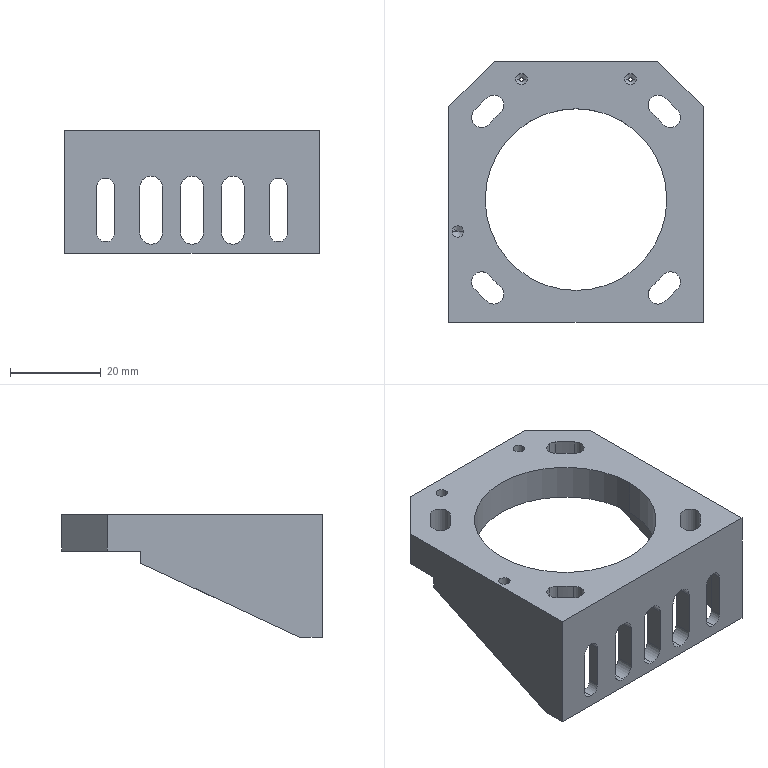NC program | NX | posted with a generic post | part box 56 x 57.4 x 27 mm
Lines 13891 to 14809 of 23725:
(ZLEVEL_PROFILE_COPY_2 , TOOL : D6JING)
N27762 T06 M6
N27764 G54
N27766 G17 G0 G90 X-22. Y20.857 B0. C0. S5000 M3
N27768 G43 Z30. H6
N27770 Z-0.1
N27772 G94 G1 X-22.627 Y21.749 F1000.
N27774 G3 X-23.171 Y22.001 R0.6
N27776 G1 X-23.2 Y21.999 F1500.
N27778 Y20.313
N27780 G3 X-22.9 Y19.793 R0.6
N27782 G1 X-22. Y19.274
N27784 G0 Y20.767 Z-0.2
N27786 G1 X-22.639 Y21.732 F1000.
N27788 G3 X-23.176 Y22. R0.6
N27790 G1 X-23.2 Y21.999 F1500.
N27792 Y20.227
N27794 G3 X-22.9 Y19.707 R0.6
N27796 G1 X-22. Y19.188
N27798 G0 Y20.77 Z-0.3
N27800 G1 X-22.537 Y21.7 F1000.
N27802 G3 X-23.057 Y22. R0.6
N27804 G1 X-23.176 F1500.
N27806 X-23.2 Y21.999
N27808 Y20.14
N27810 G3 X-22.9 Y19.621 R0.6
N27812 G1 X-22. Y19.101
N27814 G0 X-21.87 Y20.917 Z-0.4
N27816 G1 X-22.323 Y21.7 F1000.
N27818 G3 X-22.842 Y22. R0.6
N27820 G1 X-23.176 F1500.
N27822 X-23.2 Y21.999
N27824 Y20.061
N27826 G3 X-22.9 Y19.541 R0.6
N27828 G1 X-22. Y19.021
N27830 G0 X-21.654 Y20.914 Z-0.5
N27832 G1 X-22.108 Y21.7 F1000.
N27834 G3 X-22.628 Y22. R0.6
N27836 G1 X-23.176 F1500.
N27838 X-23.2 Y21.999
N27840 Y19.993
N27842 G3 X-22.9 Y19.474 R0.6
N27844 G1 X-22. Y18.954
N27846 G0 X-21.44 Y20.914 Z-0.6
N27848 G1 X-21.894 Y21.7 F1000.
N27850 G3 X-22.413 Y22. R0.6
N27852 G1 X-23.176 F1500.
N27854 X-23.2 Y21.999
N27856 Y19.933
N27858 G3 X-22.9 Y19.414 R0.6
N27860 G1 X-22. Y18.894
N27862 G0 X-21.226 Y20.914 Z-0.7
N27864 G1 X-21.679 Y21.7 F1000.
N27866 G3 X-22.199 Y22. R0.6
N27868 G1 X-23.176 F1500.
N27870 X-23.2 Y21.999
N27872 Y19.885
N27874 G3 X-22.9 Y19.365 R0.6
N27876 G1 X-22. Y18.846
N27878 G0 X-21.011 Y20.914 Z-0.8
N27880 G1 X-21.465 Y21.7 F1000.
N27882 G3 X-21.984 Y22. R0.6
N27884 G1 X-23.176 F1500.
N27886 X-23.2 Y21.999
N27888 Y19.845
N27890 G3 X-22.9 Y19.326 R0.6
N27892 G1 X-22. Y18.806
N27894 G0 X-20.797 Y20.914 Z-0.9
N27896 G1 X-21.25 Y21.7 F1000.
N27898 G3 X-21.77 Y22. R0.6
N27900 G1 X-23.176 F1500.
N27902 X-23.2 Y21.998
N27904 Y19.817
N27906 G3 X-22.9 Y19.297 R0.6
N27908 G1 X-22. Y18.778
N27910 G0 X-20.582 Y20.914 Z-1.
N27912 G1 X-21.036 Y21.7 F1000.
N27914 G3 X-21.555 Y22. R0.6
N27916 G1 X-23.176 F1500.
N27918 X-23.2 Y21.998
N27920 Y19.796
N27922 G3 X-22.9 Y19.277 R0.6
N27924 G1 X-22. Y18.757
N27926 G0 X-20.368 Y20.914 Z-1.1
N27928 G1 X-20.821 Y21.7 F1000.
N27930 G3 X-21.341 Y22. R0.6
N27932 G1 X-23.176 F1500.
N27934 X-23.2 Y21.998
N27936 Y19.786
N27938 G3 X-22.9 Y19.267 R0.6
N27940 G1 X-22. Y18.747
N27942 G0 X-20.153 Y20.914 Z-1.2
N27944 G1 X-20.607 Y21.7 F1000.
N27946 G3 X-21.127 Y22. R0.6
N27948 G1 X-23.176 F1500.
N27950 X-23.2 Y21.998
N27952 Y19.784
N27954 G3 X-22.9 Y19.264 R0.6
N27956 G1 X-22. Y18.744
N27958 G0 X-20.002 Y20.9 Z-1.3
N27960 G1 X-20.464 Y21.7 F1000.
N27962 G3 X-20.984 Y22. R0.6
N27964 G1 X-23.176 F1500.
N27966 X-23.2 Y21.998
N27968 Y19.784
N27970 G3 X-22.9 Y19.264 R0.6
N27972 G1 X-22. Y18.744
N27974 G0 X-19.98 Y20.863 Z-1.4
N27976 G1 X-20.464 Y21.7 F1000.
N27978 G3 X-20.984 Y22. R0.6
N27980 G1 X-23.176 F1500.
N27982 X-23.2 Y21.998
N27984 Y19.784
N27986 G3 X-22.9 Y19.264 R0.6
N27988 G1 X-22. Y18.744
N27990 G0 X-19.963 Y20.832 Z-1.5
N27992 G1 X-20.464 Y21.7 F1000.
N27994 G3 X-20.984 Y22. R0.6
N27996 G1 X-23.176 F1500.
N27998 X-23.2 Y21.998
N28000 Y19.784
N28002 G3 X-22.9 Y19.264 R0.6
N28004 G1 X-22. Y18.744
N28006 G0 X-19.952 Y20.813 Z-1.6
N28008 G1 X-20.464 Y21.7 F1000.
N28010 G3 X-20.984 Y22. R0.6
N28012 G1 X-23.176 F1500.
N28014 X-23.2 Y21.998
N28016 Y19.784
N28018 G3 X-22.9 Y19.264 R0.6
N28020 G1 X-22. Y18.744
N28022 G0 X-19.945 Y20.802 Z-1.7
N28024 G1 X-20.464 Y21.7 F1000.
N28026 G3 X-20.984 Y22. R0.6
N28028 G1 X-23.176 F1500.
N28030 X-23.2 Y21.998
N28032 Y19.784
N28034 G3 X-22.9 Y19.264 R0.6
N28036 G1 X-22. Y18.744
N28038 G0 X-19.944 Y20.8 Z-1.8
N28040 G1 X-20.464 Y21.7 F1000.
N28042 G3 X-20.984 Y22. R0.6
N28044 G1 X-23.176 F1500.
N28046 X-23.2 Y21.998
N28048 Y19.784
N28050 G3 X-22.9 Y19.264 R0.6
N28052 G1 X-22. Y18.744
N28054 G0 X-19.944 Y20.8 Z-1.9
N28056 G1 X-20.464 Y21.7 F1000.
N28058 G3 X-20.984 Y22. R0.6
N28060 G1 X-23.176 F1500.
N28062 X-23.2 Y21.998
N28064 Y19.784
N28066 G3 X-22.9 Y19.264 R0.6
N28068 G1 X-22. Y18.744
N28070 G0 X-19.944 Y20.8 Z-2.
N28072 G1 X-20.464 Y21.7 F1000.
N28074 G3 X-20.984 Y22. R0.6
N28076 G1 X-23.176 F1500.
N28078 X-23.2 Y21.998
N28080 Y19.784
N28082 G3 X-22.9 Y19.264 R0.6
N28084 G1 X-22. Y18.744
N28086 G0 X-19.944 Y20.8 Z-2.1
N28088 G1 X-20.464 Y21.7 F1000.
N28090 G3 X-20.984 Y22. R0.6
N28092 G1 X-23.176 F1500.
N28094 X-23.2 Y21.998
N28096 Y19.784
N28098 G3 X-22.9 Y19.264 R0.6
N28100 G1 X-22. Y18.744
N28102 G0 X-19.944 Y20.8 Z-2.2
N28104 G1 X-20.464 Y21.7 F1000.
N28106 G3 X-20.984 Y22. R0.6
N28108 G1 X-23.176 F1500.
N28110 X-23.2 Y21.998
N28112 Y19.784
N28114 G3 X-22.9 Y19.264 R0.6
N28116 G1 X-22. Y18.744
N28118 G0 X-19.944 Y20.8 Z-2.3
N28120 G1 X-20.464 Y21.7 F1000.
N28122 G3 X-20.984 Y22. R0.6
N28124 G1 X-23.176 F1500.
N28126 X-23.2 Y21.998
N28128 Y19.784
N28130 G3 X-22.9 Y19.264 R0.6
N28132 G1 X-22. Y18.744
N28134 G0 X-19.944 Y20.8 Z-2.4
N28136 G1 X-20.464 Y21.7 F1000.
N28138 G3 X-20.984 Y22. R0.6
N28140 G1 X-23.176 F1500.
N28142 X-23.2 Y21.998
N28144 Y19.784
N28146 G3 X-22.9 Y19.264 R0.6
N28148 G1 X-22. Y18.744
N28150 G0 X-19.944 Y20.8 Z-2.5
N28152 G1 X-20.464 Y21.7 F1000.
N28154 G3 X-20.984 Y22. R0.6
N28156 G1 X-23.176 F1500.
N28158 X-23.2 Y21.998
N28160 Y19.784
N28162 G3 X-22.9 Y19.264 R0.6
N28164 G1 X-22. Y18.744
N28166 G0 X-19.944 Y20.8 Z-2.6
N28168 G1 X-20.464 Y21.7 F1000.
N28170 G3 X-20.984 Y22. R0.6
N28172 G1 X-23.176 F1500.
N28174 X-23.2 Y21.998
N28176 Y19.784
N28178 G3 X-22.9 Y19.264 R0.6
N28180 G1 X-22. Y18.744
N28182 G0 X-19.944 Y20.8 Z-2.7
N28184 G1 X-20.464 Y21.7 F1000.
N28186 G3 X-20.984 Y22. R0.6
N28188 G1 X-23.176 F1500.
N28190 X-23.2 Y21.998
N28192 Y19.784
N28194 G3 X-22.9 Y19.264 R0.6
N28196 G1 X-22. Y18.744
N28198 G0 X-19.944 Y20.8 Z-2.8
N28200 G1 X-20.464 Y21.7 F1000.
N28202 G3 X-20.984 Y22. R0.6
N28204 G1 X-23.176 F1500.
N28206 X-23.2 Y21.998
N28208 Y19.784
N28210 G3 X-22.9 Y19.264 R0.6
N28212 G1 X-22. Y18.744
N28214 G0 X-19.944 Y20.8 Z-2.9
N28216 G1 X-20.464 Y21.7 F1000.
N28218 G3 X-20.984 Y22. R0.6
N28220 G1 X-23.176 F1500.
N28222 X-23.2 Y21.998
N28224 Y19.784
N28226 G3 X-22.9 Y19.264 R0.6
N28228 G1 X-22. Y18.744
N28230 G0 X-19.944 Y20.8 Z-3.
N28232 G1 X-20.464 Y21.7 F1000.
N28234 G3 X-20.984 Y22. R0.6
N28236 G1 X-23.176 F1500.
N28238 X-23.2 Y21.998
N28240 Y19.784
N28242 G3 X-22.9 Y19.264 R0.6
N28244 G1 X-22. Y18.744
N28246 G0 X-19.944 Y20.8 Z-3.1
N28248 G1 X-20.464 Y21.7 F1000.
N28250 G3 X-20.984 Y22. R0.6
N28252 G1 X-23.176 F1500.
N28254 X-23.2 Y21.998
N28256 Y19.784
N28258 G3 X-22.9 Y19.264 R0.6
N28260 G1 X-22. Y18.744
N28262 G0 X-19.944 Y20.8 Z-3.2
N28264 G1 X-20.464 Y21.7 F1000.
N28266 G3 X-20.984 Y22. R0.6
N28268 G1 X-23.176 F1500.
N28270 X-23.2 Y21.998
N28272 Y19.784
N28274 G3 X-22.9 Y19.264 R0.6
N28276 G1 X-22. Y18.744
N28278 G0 X-19.944 Y20.8 Z-3.3
N28280 G1 X-20.464 Y21.7 F1000.
N28282 G3 X-20.984 Y22. R0.6
N28284 G1 X-23.176 F1500.
N28286 X-23.2 Y21.998
N28288 Y19.784
N28290 G3 X-22.9 Y19.264 R0.6
N28292 G1 X-22. Y18.744
N28294 G0 X-19.944 Y20.8 Z-3.4
N28296 G1 X-20.464 Y21.7 F1000.
N28298 G3 X-20.984 Y22. R0.6
N28300 G1 X-23.176 F1500.
N28302 X-23.2 Y21.998
N28304 Y19.784
N28306 G3 X-22.9 Y19.264 R0.6
N28308 G1 X-22. Y18.744
N28310 G0 X-19.944 Y20.8 Z-3.5
N28312 G1 X-20.464 Y21.7 F1000.
N28314 G3 X-20.984 Y22. R0.6
N28316 G1 X-23.176 F1500.
N28318 X-23.2 Y21.998
N28320 Y19.784
N28322 G3 X-22.9 Y19.264 R0.6
N28324 G1 X-22. Y18.744
N28326 G0 X-19.944 Y20.8 Z-3.6
N28328 G1 X-20.464 Y21.7 F1000.
N28330 G3 X-20.984 Y22. R0.6
N28332 G1 X-23.176 F1500.
N28334 X-23.2 Y21.998
N28336 Y19.784
N28338 G3 X-22.9 Y19.264 R0.6
N28340 G1 X-22. Y18.744
N28342 G0 X-19.944 Y20.8 Z-3.7
N28344 G1 X-20.464 Y21.7 F1000.
N28346 G3 X-20.984 Y22. R0.6
N28348 G1 X-23.176 F1500.
N28350 X-23.2 Y21.998
N28352 Y19.784
N28354 G3 X-22.9 Y19.264 R0.6
N28356 G1 X-22. Y18.744
N28358 G0 X-19.944 Y20.8 Z-3.8
N28360 G1 X-20.464 Y21.7 F1000.
N28362 G3 X-20.984 Y22. R0.6
N28364 G1 X-23.176 F1500.
N28366 X-23.2 Y21.998
N28368 Y19.784
N28370 G3 X-22.9 Y19.264 R0.6
N28372 G1 X-22. Y18.744
N28374 G0 X-19.944 Y20.8 Z-3.9
N28376 G1 X-20.464 Y21.7 F1000.
N28378 G3 X-20.984 Y22. R0.6
N28380 G1 X-23.176 F1500.
N28382 X-23.2 Y21.998
N28384 Y19.784
N28386 G3 X-22.9 Y19.264 R0.6
N28388 G1 X-22. Y18.744
N28390 G0 X-19.944 Y20.8 Z-4.
N28392 G1 X-20.464 Y21.7 F1000.
N28394 G3 X-20.984 Y22. R0.6
N28396 G1 X-23.176 F1500.
N28398 X-23.2 Y21.998
N28400 Y19.784
N28402 G3 X-22.9 Y19.264 R0.6
N28404 G1 X-22. Y18.744
N28406 G0 X-19.944 Y20.8 Z-4.1
N28408 G1 X-20.464 Y21.7 F1000.
N28410 G3 X-20.984 Y22. R0.6
N28412 G1 X-23.176 F1500.
N28414 X-23.2 Y21.998
N28416 Y19.784
N28418 G3 X-22.9 Y19.264 R0.6
N28420 G1 X-22. Y18.744
N28422 G0 X-19.944 Y20.8 Z-4.2
N28424 G1 X-20.464 Y21.7 F1000.
N28426 G3 X-20.984 Y22. R0.6
N28428 G1 X-23.176 F1500.
N28430 X-23.2 Y21.998
N28432 Y19.784
N28434 G3 X-22.9 Y19.264 R0.6
N28436 G1 X-22. Y18.744
N28438 G0 X-19.944 Y20.8 Z-4.3
N28440 G1 X-20.464 Y21.7 F1000.
N28442 G3 X-20.984 Y22. R0.6
N28444 G1 X-23.176 F1500.
N28446 X-23.2 Y21.998
N28448 Y19.784
N28450 G3 X-22.9 Y19.264 R0.6
N28452 G1 X-22. Y18.744
N28454 G0 X-19.944 Y20.8 Z-4.4
N28456 G1 X-20.464 Y21.7 F1000.
N28458 G3 X-20.984 Y22. R0.6
N28460 G1 X-23.176 F1500.
N28462 X-23.2 Y21.998
N28464 Y19.784
N28466 G3 X-22.9 Y19.264 R0.6
N28468 G1 X-22. Y18.744
N28470 G0 X-19.944 Y20.8 Z-4.5
N28472 G1 X-20.464 Y21.7 F1000.
N28474 G3 X-20.984 Y22. R0.6
N28476 G1 X-23.176 F1500.
N28478 X-23.2 Y21.998
N28480 Y19.784
N28482 G3 X-22.9 Y19.264 R0.6
N28484 G1 X-22. Y18.744
N28486 G0 X-19.944 Y20.8 Z-4.6
N28488 G1 X-20.464 Y21.7 F1000.
N28490 G3 X-20.984 Y22. R0.6
N28492 G1 X-23.176 F1500.
N28494 X-23.2 Y21.998
N28496 Y19.784
N28498 G3 X-22.9 Y19.264 R0.6
N28500 G1 X-22. Y18.744
N28502 G0 X-19.944 Y20.8 Z-4.7
N28504 G1 X-20.464 Y21.7 F1000.
N28506 G3 X-20.984 Y22. R0.6
N28508 G1 X-23.176 F1500.
N28510 X-23.2 Y21.998
N28512 Y19.784
N28514 G3 X-22.9 Y19.264 R0.6
N28516 G1 X-22. Y18.744
N28518 G0 X-19.944 Y20.8 Z-4.8
N28520 G1 X-20.464 Y21.7 F1000.
N28522 G3 X-20.984 Y22. R0.6
N28524 G1 X-23.176 F1500.
N28526 X-23.2 Y21.998
N28528 Y19.784
N28530 G3 X-22.9 Y19.264 R0.6
N28532 G1 X-22. Y18.744
N28534 G0 X-19.944 Y20.8 Z-4.9
N28536 G1 X-20.464 Y21.7 F1000.
N28538 G3 X-20.984 Y22. R0.6
N28540 G1 X-23.176 F1500.
N28542 X-23.2 Y21.998
N28544 Y19.784
N28546 G3 X-22.9 Y19.264 R0.6
N28548 G1 X-22. Y18.744
N28550 G0 X-19.944 Y20.8 Z-5.
N28552 G1 X-20.464 Y21.7 F1000.
N28554 G3 X-20.984 Y22. R0.6
N28556 G1 X-23.176 F1500.
N28558 X-23.2 Y21.998
N28560 Y19.784
N28562 G3 X-22.9 Y19.264 R0.6
N28564 G1 X-22. Y18.744
N28566 G0 X-19.944 Y20.8 Z-5.1
N28568 G1 X-20.464 Y21.7 F1000.
N28570 G3 X-20.984 Y22. R0.6
N28572 G1 X-23.176 F1500.
N28574 X-23.2 Y21.998
N28576 Y19.784
N28578 G3 X-22.9 Y19.264 R0.6
N28580 G1 X-22. Y18.744
N28582 G0 X-19.944 Y20.8 Z-5.2
N28584 G1 X-20.464 Y21.7 F1000.
N28586 G3 X-20.984 Y22. R0.6
N28588 G1 X-23.176 F1500.
N28590 X-23.2 Y21.998
N28592 Y19.784
N28594 G3 X-22.9 Y19.264 R0.6
N28596 G1 X-22. Y18.744
N28598 G0 X-19.944 Y20.8 Z-5.3
N28600 G1 X-20.464 Y21.7 F1000.
N28602 G3 X-20.984 Y22. R0.6
N28604 G1 X-23.176 F1500.
N28606 X-23.2 Y21.998
N28608 Y19.784
N28610 G3 X-22.9 Y19.264 R0.6
N28612 G1 X-22. Y18.744
N28614 G0 X-19.944 Y20.8 Z-5.4
N28616 G1 X-20.464 Y21.7 F1000.
N28618 G3 X-20.984 Y22. R0.6
N28620 G1 X-23.176 F1500.
N28622 X-23.2 Y21.998
N28624 Y19.784
N28626 G3 X-22.9 Y19.264 R0.6
N28628 G1 X-22. Y18.744
N28630 G0 X-19.944 Y20.8 Z-5.5
N28632 G1 X-20.464 Y21.7 F1000.
N28634 G3 X-20.984 Y22. R0.6
N28636 G1 X-23.176 F1500.
N28638 X-23.2 Y21.998
N28640 Y19.784
N28642 G3 X-22.9 Y19.264 R0.6
N28644 G1 X-22. Y18.744
N28646 G0 X-19.944 Y20.8 Z-5.6
N28648 G1 X-20.464 Y21.7 F1000.
N28650 G3 X-20.984 Y22. R0.6
N28652 G1 X-23.176 F1500.
N28654 X-23.2 Y21.998
N28656 Y19.784
N28658 G3 X-22.9 Y19.264 R0.6
N28660 G1 X-22. Y18.744
N28662 G0 X-19.944 Y20.8 Z-5.7
N28664 G1 X-20.464 Y21.7 F1000.
N28666 G3 X-20.984 Y22. R0.6
N28668 G1 X-23.176 F1500.
N28670 X-23.2 Y21.998
N28672 Y19.784
N28674 G3 X-22.9 Y19.264 R0.6
N28676 G1 X-22. Y18.744
N28678 G0 X-19.944 Y20.8 Z-5.8
N28680 G1 X-20.464 Y21.7 F1000.
N28682 G3 X-20.984 Y22. R0.6
N28684 G1 X-23.176 F1500.
N28686 X-23.2 Y21.998
N28688 Y19.784
N28690 G3 X-22.9 Y19.264 R0.6
N28692 G1 X-22. Y18.744
N28694 G0 X-19.944 Y20.8 Z-5.9
N28696 G1 X-20.464 Y21.7 F1000.
N28698 G3 X-20.984 Y22. R0.6
N28700 G1 X-23.176 F1500.
N28702 X-23.2 Y21.998
N28704 Y19.784
N28706 G3 X-22.9 Y19.264 R0.6
N28708 G1 X-22. Y18.744
N28710 G0 X-19.944 Y20.8 Z-6.
N28712 G1 X-20.464 Y21.7 F1000.
N28714 G3 X-20.984 Y22. R0.6
N28716 G1 X-23.176 F1500.
N28718 X-23.2 Y21.998
N28720 Y19.784
N28722 G3 X-22.9 Y19.264 R0.6
N28724 G1 X-22. Y18.744
N28726 G0 X-19.944 Y20.8 Z-6.1
N28728 G1 X-20.464 Y21.7 F1000.
N28730 G3 X-20.984 Y22. R0.6
N28732 G1 X-23.176 F1500.
N28734 X-23.2 Y21.998
N28736 Y19.784
N28738 G3 X-22.9 Y19.264 R0.6
N28740 G1 X-22. Y18.744
N28742 G0 X-19.944 Y20.8 Z-6.2
N28744 G1 X-20.464 Y21.7 F1000.
N28746 G3 X-20.984 Y22. R0.6
N28748 G1 X-23.176 F1500.
N28750 X-23.2 Y21.998
N28752 Y19.784
N28754 G3 X-22.9 Y19.264 R0.6
N28756 G1 X-22. Y18.744
N28758 G0 X-19.944 Y20.8 Z-6.3
N28760 G1 X-20.464 Y21.7 F1000.
N28762 G3 X-20.984 Y22. R0.6
N28764 G1 X-23.176 F1500.
N28766 X-23.2 Y21.998
N28768 Y19.784
N28770 G3 X-22.9 Y19.264 R0.6
N28772 G1 X-22. Y18.744
N28774 G0 X-19.944 Y20.8 Z-6.4
N28776 G1 X-20.464 Y21.7 F1000.
N28778 G3 X-20.984 Y22. R0.6
N28780 G1 X-23.176 F1500.
N28782 X-23.2 Y21.998
N28784 Y19.784
N28786 G3 X-22.9 Y19.264 R0.6
N28788 G1 X-22. Y18.744
N28790 G0 X-19.944 Y20.8 Z-6.5
N28792 G1 X-20.464 Y21.7 F1000.
N28794 G3 X-20.984 Y22. R0.6
N28796 G1 X-23.176 F1500.
N28798 X-23.2 Y21.998
N28800 Y19.784
N28802 G3 X-22.9 Y19.264 R0.6
N28804 G1 X-22. Y18.744
N28806 G0 X-19.944 Y20.8 Z-6.6
N28808 G1 X-20.464 Y21.7 F1000.
N28810 G3 X-20.984 Y22. R0.6
N28812 G1 X-23.176 F1500.
N28814 X-23.2 Y21.998
N28816 Y19.784
N28818 G3 X-22.9 Y19.264 R0.6
N28820 G1 X-22. Y18.744
N28822 G0 X-19.944 Y20.8 Z-6.7
N28824 G1 X-20.464 Y21.7 F1000.
N28826 G3 X-20.984 Y22. R0.6
N28828 G1 X-23.176 F1500.
N28830 X-23.2 Y21.998
N28832 Y19.784
N28834 G3 X-22.9 Y19.264 R0.6
N28836 G1 X-22. Y18.744
N28838 G0 X-19.944 Y20.8 Z-6.8
N28840 G1 X-20.464 Y21.7 F1000.
N28842 G3 X-20.984 Y22. R0.6
N28844 G1 X-23.176 F1500.
N28846 X-23.2 Y21.998
N28848 Y19.784
N28850 G3 X-22.9 Y19.264 R0.6
N28852 G1 X-22. Y18.744
N28854 G0 X-19.944 Y20.8 Z-6.9
N28856 G1 X-20.464 Y21.7 F1000.
N28858 G3 X-20.984 Y22. R0.6
N28860 G1 X-23.176 F1500.
N28862 X-23.2 Y21.998
N28864 Y19.784
N28866 G3 X-22.9 Y19.264 R0.6
N28868 G1 X-22. Y18.744
N28870 G0 X-19.944 Y20.8 Z-7.
N28872 G1 X-20.464 Y21.7 F1000.
N28874 G3 X-20.984 Y22. R0.6
N28876 G1 X-23.176 F1500.
N28878 X-23.2 Y21.998
N28880 Y19.784
N28882 G3 X-22.9 Y19.264 R0.6
N28884 G1 X-22. Y18.744
N28886 G0 X-19.944 Y20.8 Z-7.1
N28888 G1 X-20.464 Y21.7 F1000.
N28890 G3 X-20.984 Y22. R0.6
N28892 G1 X-23.176 F1500.
N28894 X-23.2 Y21.998
N28896 Y19.784
N28898 G3 X-22.9 Y19.264 R0.6
N28900 G1 X-22. Y18.744
N28902 G0 X-19.944 Y20.8 Z-7.2
N28904 G1 X-20.464 Y21.7 F1000.
N28906 G3 X-20.984 Y22. R0.6
N28908 G1 X-23.176 F1500.
N28910 X-23.2 Y21.998
N28912 Y19.784
N28914 G3 X-22.9 Y19.264 R0.6
N28916 G1 X-22. Y18.744
N28918 G0 X-19.944 Y20.8 Z-7.3
N28920 G1 X-20.464 Y21.7 F1000.
N28922 G3 X-20.984 Y22. R0.6
N28924 G1 X-23.176 F1500.
N28926 X-23.2 Y21.998
N28928 Y19.784
N28930 G3 X-22.9 Y19.264 R0.6
N28932 G1 X-22. Y18.744
N28934 G0 X-19.944 Y20.8 Z-7.4
N28936 G1 X-20.464 Y21.7 F1000.
N28938 G3 X-20.984 Y22. R0.6
N28940 G1 X-23.176 F1500.
N28942 X-23.2 Y21.998
N28944 Y19.784
N28946 G3 X-22.9 Y19.264 R0.6
N28948 G1 X-22. Y18.744
N28950 G0 X-19.944 Y20.8 Z-7.5
N28952 G1 X-20.464 Y21.7 F1000.
N28954 G3 X-20.984 Y22. R0.6
N28956 G1 X-23.176 F1500.
N28958 X-23.2 Y21.998
N28960 Y19.784
N28962 G3 X-22.9 Y19.264 R0.6
N28964 G1 X-22. Y18.744
N28966 G0 X-19.944 Y20.8 Z-7.6
N28968 G1 X-20.464 Y21.7 F1000.
N28970 G3 X-20.984 Y22. R0.6
N28972 G1 X-23.176 F1500.
N28974 X-23.2 Y21.998
N28976 Y19.784
N28978 G3 X-22.9 Y19.264 R0.6
N28980 G1 X-22. Y18.744
N28982 G0 X-19.944 Y20.8 Z-7.7
N28984 G1 X-20.464 Y21.7 F1000.
N28986 G3 X-20.984 Y22. R0.6
N28988 G1 X-23.176 F1500.
N28990 X-23.2 Y21.998
N28992 Y19.784
N28994 G3 X-22.9 Y19.264 R0.6
N28996 G1 X-22. Y18.744
N28998 G0 X-19.944 Y20.8 Z-7.8
N29000 G1 X-20.464 Y21.7 F1000.
N29002 G3 X-20.984 Y22. R0.6
N29004 G1 X-23.176 F1500.
N29006 X-23.2 Y21.998
N29008 Y19.784
N29010 G3 X-22.9 Y19.264 R0.6
N29012 G1 X-22. Y18.744
N29014 G0 X-19.944 Y20.8 Z-7.9
N29016 G1 X-20.464 Y21.7 F1000.
N29018 G3 X-20.984 Y22. R0.6
N29020 G1 X-23.176 F1500.
N29022 X-23.2 Y21.998
N29024 Y19.784
N29026 G3 X-22.9 Y19.264 R0.6
N29028 G1 X-22. Y18.744
N29030 G0 X-19.944 Y20.8 Z-8.
N29032 G1 X-20.464 Y21.7 F1000.
N29034 G3 X-20.984 Y22. R0.6
N29036 G1 X-23.176 F1500.
N29038 X-23.2 Y21.998
N29040 Y19.784
N29042 G3 X-22.9 Y19.264 R0.6
N29044 G1 X-22. Y18.744
N29046 G0 X-19.944 Y20.8 Z-8.1
N29048 G1 X-20.464 Y21.7 F1000.
N29050 G3 X-20.984 Y22. R0.6
N29052 G1 X-23.176 F1500.
N29054 X-23.2 Y21.998
N29056 Y19.784
N29058 G3 X-22.9 Y19.264 R0.6
N29060 G1 X-22. Y18.744
N29062 G0 X-19.944 Y20.8 Z-8.2
N29064 G1 X-20.464 Y21.7 F1000.
N29066 G3 X-20.984 Y22. R0.6
N29068 G1 X-23.176 F1500.
N29070 X-23.2 Y21.998
N29072 Y19.784
N29074 G3 X-22.9 Y19.264 R0.6
N29076 G1 X-22. Y18.744
N29078 G0 X-19.944 Y20.8 Z-8.3
N29080 G1 X-20.464 Y21.7 F1000.
N29082 G3 X-20.984 Y22. R0.6
N29084 G1 X-23.176 F1500.
N29086 X-23.2 Y21.998
N29088 Y19.784
N29090 G3 X-22.9 Y19.264 R0.6
N29092 G1 X-22. Y18.744
N29094 G0 X-19.944 Y20.8 Z-8.4
N29096 G1 X-20.464 Y21.7 F1000.
N29098 G3 X-20.984 Y22. R0.6
N29100 G1 X-23.176 F1500.
N29102 X-23.2 Y21.998
N29104 Y19.784
N29106 G3 X-22.9 Y19.264 R0.6
N29108 G1 X-22. Y18.744
N29110 G0 X-19.944 Y20.8 Z-8.5
N29112 G1 X-20.464 Y21.7 F1000.
N29114 G3 X-20.984 Y22. R0.6
N29116 G1 X-23.176 F1500.
N29118 X-23.2 Y21.998
N29120 Y19.784
N29122 G3 X-22.9 Y19.264 R0.6
N29124 G1 X-22. Y18.744
N29126 G0 X-19.944 Y20.8 Z-8.6
N29128 G1 X-20.464 Y21.7 F1000.
N29130 G3 X-20.984 Y22. R0.6
N29132 G1 X-23.176 F1500.
N29134 X-23.2 Y21.998
N29136 Y19.784
N29138 G3 X-22.9 Y19.264 R0.6
N29140 G1 X-22. Y18.744
N29142 G0 X-19.944 Y20.8 Z-8.7
N29144 G1 X-20.464 Y21.7 F1000.
N29146 G3 X-20.984 Y22. R0.6
N29148 G1 X-23.176 F1500.
N29150 X-23.2 Y21.998
N29152 Y19.784
N29154 G3 X-22.9 Y19.264 R0.6
N29156 G1 X-22. Y18.744
N29158 G0 X-19.944 Y20.8 Z-8.8
N29160 G1 X-20.464 Y21.7 F1000.
N29162 G3 X-20.984 Y22. R0.6
N29164 G1 X-23.176 F1500.
N29166 X-23.2 Y21.998
N29168 Y19.784
N29170 G3 X-22.9 Y19.264 R0.6
N29172 G1 X-22. Y18.744
N29174 G0 X-19.944 Y20.8 Z-8.9
N29176 G1 X-20.464 Y21.7 F1000.
N29178 G3 X-20.984 Y22. R0.6
N29180 G1 X-23.176 F1500.
N29182 X-23.2 Y21.998
N29184 Y19.784
N29186 G3 X-22.9 Y19.264 R0.6
N29188 G1 X-22. Y18.744
N29190 G0 X-19.944 Y20.8 Z-9.
N29192 G1 X-20.464 Y21.7 F1000.
N29194 G3 X-20.984 Y22. R0.6
N29196 G1 X-23.176 F1500.
N29198 X-23.2 Y21.998
N29200 Y19.784
N29202 G3 X-22.9 Y19.264 R0.6
N29204 G1 X-22. Y18.744
N29206 G0 X-19.944 Y20.8 Z-9.1
N29208 G1 X-20.464 Y21.7 F1000.
N29210 G3 X-20.984 Y22. R0.6
N29212 G1 X-23.176 F1500.
N29214 X-23.2 Y21.998
N29216 Y19.784
N29218 G3 X-22.9 Y19.264 R0.6
N29220 G1 X-22. Y18.744
N29222 G0 X-19.944 Y20.8 Z-9.2
N29224 G1 X-20.464 Y21.7 F1000.
N29226 G3 X-20.984 Y22. R0.6
N29228 G1 X-23.176 F1500.
N29230 X-23.2 Y21.998
N29232 Y19.784
N29234 G3 X-22.9 Y19.264 R0.6
N29236 G1 X-22. Y18.744
N29238 G0 X-19.944 Y20.8 Z-9.3
N29240 G1 X-20.464 Y21.7 F1000.
N29242 G3 X-20.984 Y22. R0.6
N29244 G1 X-23.176 F1500.
N29246 X-23.2 Y21.998
N29248 Y19.784
N29250 G3 X-22.9 Y19.264 R0.6
N29252 G1 X-22. Y18.744
N29254 G0 X-19.944 Y20.8 Z-9.4
N29256 G1 X-20.464 Y21.7 F1000.
N29258 G3 X-20.984 Y22. R0.6
N29260 G1 X-23.176 F1500.
N29262 X-23.2 Y21.998
N29264 Y19.784
N29266 G3 X-22.9 Y19.264 R0.6
N29268 G1 X-22. Y18.744
N29270 G0 X-19.944 Y20.8 Z-9.5
N29272 G1 X-20.464 Y21.7 F1000.
N29274 G3 X-20.984 Y22. R0.6
N29276 G1 X-23.176 F1500.
N29278 X-23.2 Y21.998
N29280 Y19.784
N29282 G3 X-22.9 Y19.264 R0.6
N29284 G1 X-22. Y18.744
N29286 G0 X-19.944 Y20.8 Z-9.6
N29288 G1 X-20.464 Y21.7 F1000.
N29290 G3 X-20.984 Y22. R0.6
N29292 G1 X-23.176 F1500.
N29294 X-23.2 Y21.998
N29296 Y19.784
N29298 G3 X-22.9 Y19.264 R0.6
N29300 G1 X-22. Y18.744
N29302 G0 X-19.944 Y20.8 Z-9.7
N29304 G1 X-20.464 Y21.7 F1000.
N29306 G3 X-20.984 Y22. R0.6
N29308 G1 X-23.176 F1500.
N29310 X-23.2 Y21.998
N29312 Y19.784
N29314 G3 X-22.9 Y19.264 R0.6
N29316 G1 X-22. Y18.744
N29318 G0 X-19.944 Y20.8 Z-9.8
N29320 G1 X-20.464 Y21.7 F1000.
N29322 G3 X-20.984 Y22. R0.6
N29324 G1 X-23.176 F1500.
N29326 X-23.2 Y21.998
N29328 Y19.784
N29330 G3 X-22.9 Y19.264 R0.6
N29332 G1 X-22. Y18.744
N29334 G0 X-19.944 Y20.8 Z-9.9
N29336 G1 X-20.464 Y21.7 F1000.
N29338 G3 X-20.984 Y22. R0.6
N29340 G1 X-23.176 F1500.
N29342 X-23.2 Y21.998
N29344 Y19.784
N29346 G3 X-22.9 Y19.264 R0.6
N29348 G1 X-22. Y18.744
N29350 G0 X-19.944 Y20.8 Z-10.
N29352 G1 X-20.464 Y21.7 F1000.
N29354 G3 X-20.984 Y22. R0.6
N29356 G1 X-23.176 F1500.
N29358 X-23.2 Y21.998
N29360 Y19.784
N29362 G3 X-22.9 Y19.264 R0.6
N29364 G1 X-22. Y18.744
N29366 G0 X-19.944 Y20.8 Z-10.1
N29368 G1 X-20.464 Y21.7 F1000.
N29370 G3 X-20.984 Y22. R0.6
N29372 G1 X-23.176 F1500.
N29374 X-23.2 Y21.998
N29376 Y19.784
N29378 G3 X-22.9 Y19.264 R0.6
N29380 G1 X-22. Y18.744
N29382 G0 X-19.944 Y20.8 Z-10.2
N29384 G1 X-20.464 Y21.7 F1000.
N29386 G3 X-20.984 Y22. R0.6
N29388 G1 X-23.176 F1500.
N29390 X-23.2 Y21.998
N29392 Y19.784
N29394 G3 X-22.9 Y19.264 R0.6
N29396 G1 X-22. Y18.744
N29398 G0 X-19.944 Y20.8 Z-10.3
N29400 G1 X-20.464 Y21.7 F1000.
N29402 G3 X-20.984 Y22. R0.6
N29404 G1 X-23.176 F1500.
N29406 X-23.2 Y21.998
N29408 Y19.784
N29410 G3 X-22.9 Y19.264 R0.6
N29412 G1 X-22. Y18.744
N29414 G0 X-19.944 Y20.8 Z-10.4
N29416 G1 X-20.464 Y21.7 F1000.
N29418 G3 X-20.984 Y22. R0.6
N29420 G1 X-23.176 F1500.
N29422 X-23.2 Y21.998
N29424 Y19.784
N29426 G3 X-22.9 Y19.264 R0.6
N29428 G1 X-22. Y18.744
N29430 G0 X-19.944 Y20.8 Z-10.5
N29432 G1 X-20.464 Y21.7 F1000.
N29434 G3 X-20.984 Y22. R0.6
N29436 G1 X-23.176 F1500.
N29438 X-23.2 Y21.998
N29440 Y19.784
N29442 G3 X-22.9 Y19.264 R0.6
N29444 G1 X-22. Y18.744
N29446 G0 X-19.944 Y20.8 Z-10.6
N29448 G1 X-20.464 Y21.7 F1000.
N29450 G3 X-20.984 Y22. R0.6
N29452 G1 X-23.176 F1500.
N29454 X-23.2 Y21.998
N29456 Y19.784
N29458 G3 X-22.9 Y19.264 R0.6
N29460 G1 X-22. Y18.744
N29462 G0 X-19.944 Y20.8 Z-10.7
N29464 G1 X-20.464 Y21.7 F1000.
N29466 G3 X-20.984 Y22. R0.6
N29468 G1 X-23.176 F1500.
N29470 X-23.2 Y21.998
N29472 Y19.784
N29474 G3 X-22.9 Y19.264 R0.6
N29476 G1 X-22. Y18.744
N29478 G0 X-19.944 Y20.8 Z-10.8
N29480 G1 X-20.464 Y21.7 F1000.
N29482 G3 X-20.984 Y22. R0.6
N29484 G1 X-23.176 F1500.
N29486 X-23.2 Y21.998
N29488 Y19.784
N29490 G3 X-22.9 Y19.264 R0.6
N29492 G1 X-22. Y18.744
N29494 G0 X-19.944 Y20.8 Z-10.9
N29496 G1 X-20.464 Y21.7 F1000.
N29498 G3 X-20.984 Y22. R0.6
N29500 G1 X-23.176 F1500.
N29502 X-23.2 Y21.998
N29504 Y19.784
N29506 G3 X-22.9 Y19.264 R0.6
N29508 G1 X-22. Y18.744
N29510 G0 X-19.944 Y20.8 Z-11.
N29512 G1 X-20.464 Y21.7 F1000.
N29514 G3 X-20.984 Y22. R0.6
N29516 G1 X-23.176 F1500.
N29518 X-23.2 Y21.998
N29520 Y19.784
N29522 G3 X-22.9 Y19.264 R0.6
N29524 G1 X-22. Y18.744
N29526 G0 X-19.944 Y20.8 Z-11.1
N29528 G1 X-20.464 Y21.7 F1000.
N29530 G3 X-20.984 Y22. R0.6
N29532 G1 X-23.176 F1500.
N29534 X-23.2 Y21.998
N29536 Y19.784
N29538 G3 X-22.9 Y19.264 R0.6
N29540 G1 X-22. Y18.744
N29542 G0 X-19.944 Y20.8 Z-11.2
N29544 G1 X-20.464 Y21.7 F1000.
N29546 G3 X-20.984 Y22. R0.6
N29548 G1 X-23.176 F1500.
N29550 X-23.2 Y21.998
N29552 Y19.784
N29554 G3 X-22.9 Y19.264 R0.6
N29556 G1 X-22. Y18.744
N29558 G0 X-19.944 Y20.8 Z-11.3
N29560 G1 X-20.464 Y21.7 F1000.
N29562 G3 X-20.984 Y22. R0.6
N29564 G1 X-23.176 F1500.
N29566 X-23.2 Y21.998
N29568 Y19.784
N29570 G3 X-22.9 Y19.264 R0.6
N29572 G1 X-22. Y18.744
N29574 G0 X-19.944 Y20.8 Z-11.4
N29576 G1 X-20.464 Y21.7 F1000.
N29578 G3 X-20.984 Y22. R0.6
N29580 G1 X-23.176 F1500.
N29582 X-23.2 Y21.998
N29584 Y19.784
N29586 G3 X-22.9 Y19.264 R0.6
N29588 G1 X-22. Y18.744
N29590 G0 X-19.944 Y20.8 Z-11.5
N29592 G1 X-20.464 Y21.7 F1000.